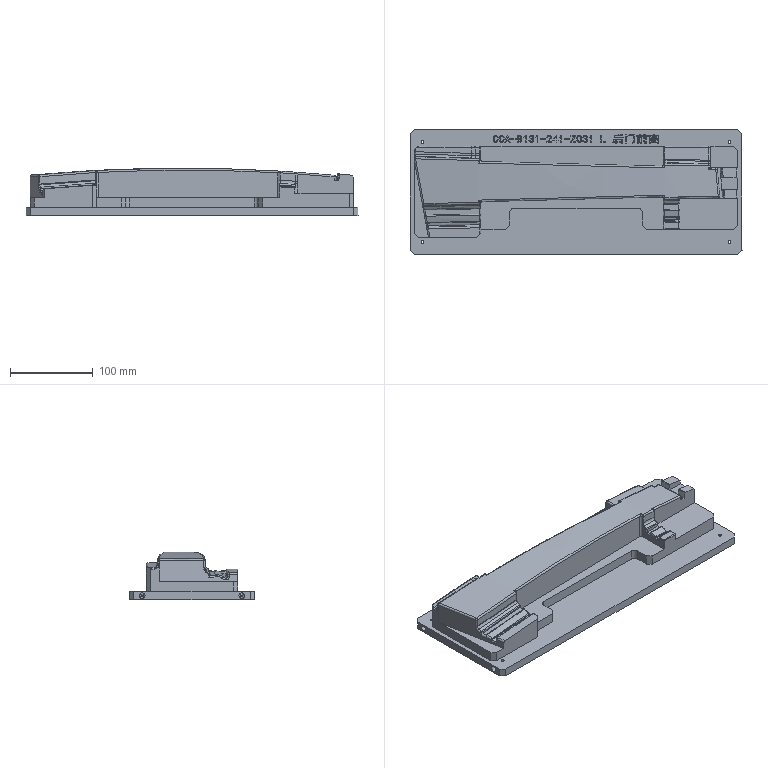NC program | NX | posted with a generic post | part box 400 x 150 x 57.494 mm
Lines 14042 to 16235 of 16235, first 2095 of 2182 lines:
(B3 , TOOL : D10)
N28076 M6
N28078 G54
N28080 G17 G0 G90 X-94.5 Y-54.975 S3500 M3
N28082 G43 Z69.994 H0
N28084 Y-54.994 Z24.994
N28086 G94 G1 Y-54.995 Z21.994 F1000.
N28088 Y-44.995 Z21.99
N28090 X-109.
N28092 Y-17.587 Z21.978
N28094 X99. Y-12.141 Z21.976
N28096 Y-43.995 Z21.989
N28098 X98.988 Y-44.499 Z21.99
N28100 X99.072 Y-44.995
N28102 X85.
N28104 X80. Y-39.995 Z21.988
N28106 Y-19.995 Z21.979
N28108 X84.348 Y-17.526 Z21.978
N28110 X94. Y-17.273
N28112 Y-39.995 Z21.988
N28114 X87.071
N28116 X85. Y-37.924 Z21.987
N28118 Y-19.995 Z21.979
N28120 X84.956 Y-19.133
N28122 X84.735 Y-18.297
N28124 X84.348 Y-17.526 Z21.978
N28126 X89.5 Y-21.893 Z21.98
N28128 Y-35.495 Z21.986
N28130 Y-21.893 Z21.98
N28132 X84.348 Y-17.526 Z21.978
N28134 X80. Y-19.995 Z21.979
N28136 X-80.
N28138 Y-39.995 Z21.988
N28140 X-85. Y-44.995 Z21.99
N28142 X-94.5
N28144 Y-39.995 Z21.988
N28146 X-104.
N28148 Y-22.458 Z21.98
N28150 X-85. Y-21.961
N28152 Y-37.924 Z21.987
N28154 X-87.071 Y-39.995 Z21.988
N28156 X-94.5
N28158 Y-34.995 Z21.986
N28160 X-99.
N28162 Y-27.329 Z21.982
N28164 X-90. Y-27.093
N28166 Y-34.995 Z21.986
N28168 X-94.5
N28170 Y-54.995 Z21.994
N28172 Y-54.994 Z24.994
N28174 G0 Y-54.975 Z69.994
(B4 , TOOL : D10)
N28176 X163.
N28178 Y-54.992 Z29.994
N28180 G1 Y-54.993 Z26.994
N28182 Y-44.993 Z26.99
N28184 X130.928
N28186 X131.012 Y-44.496
N28188 X131. Y-43.993 Z26.989
N28190 Y-13.371 Z26.977
N28192 X195.
N28194 Y-39.993 Z26.988
N28196 X190. Y-44.993 Z26.99
N28198 X163.
N28200 Y-39.993 Z26.988
N28202 X136.
N28204 Y-18.371 Z26.979
N28206 X190.
N28208 Y-37.922 Z26.987
N28210 X187.929 Y-39.993 Z26.988
N28212 X163.
N28214 Y-34.993 Z26.986
N28216 X141.
N28218 Y-23.371 Z26.981
N28220 X185.
N28222 Y-34.993 Z26.986
N28224 X163.
N28226 Y-29.993 Z26.984
N28228 X146.
N28230 Y-28.371 Z26.983
N28232 X180.
N28234 Y-29.993 Z26.984
N28236 X163.
N28238 Y-54.993 Z26.994
N28240 Y-54.992 Z29.994
N28242 G0 Y-54.975 Z69.994
(B5 , TOOL : D10)
N28244 X-205. Y-45.746
N28246 Z69.99
N28248 Y-45.765 Z24.99
N28250 G1 Y-45.766 Z21.99
N28252 X-195.
N28254 Y6.162 Z21.969
N28256 X-183.802 Y-54.995 Z21.994
N28258 X-190.
N28260 X-195. Y-49.995 Z21.992
N28262 Y-45.766 Z21.99
N28264 X-190.5
N28266 Y-43.4 Z21.989
N28268 X-189.44 Y-49.191 Z21.991
N28270 X-190.5 Y-48.131
N28272 Y-45.766 Z21.99
N28274 X-205.
N28276 Y-45.765 Z24.99
N28278 G0 Y-45.746 Z69.99
(B6 , TOOL : D10)
N28280 X181.5 Y65.146
N28282 Z69.944
N28284 Y65.132 Z35.444
N28286 G1 Y65.131 Z32.444
N28288 Y55.131 Z32.449
N28290 X190.
N28292 X195. Y50.131 Z32.451
N28294 Y35.131 Z32.457
N28296 X168.
N28298 Y53.131 Z32.449
N28300 X168.002 Y53.806
N28302 X167.916 Y54.477
N28304 X167.746 Y55.131
N28306 X181.5
N28308 Y50.131 Z32.451
N28310 X187.929
N28312 X190. Y48.06 Z32.452
N28314 Y40.131 Z32.455
N28316 X173.
N28318 Y50.131 Z32.451
N28320 X181.5
N28322 Y45.131 Z32.453
N28324 X185.
N28326 X178.
N28328 X181.5
N28330 Y65.131 Z32.444
N28332 Y65.132 Z35.444
N28334 G0 Y65.146 Z69.944
(B7 , TOOL : D10)
N28336 X-5.
N28338 Y65.132 Z35.444
N28340 G1 Y65.131 Z32.444
N28342 Y55.131 Z32.449
N28344 X99.254
N28346 X99.084 Y54.477
N28348 X98.998 Y53.806
N28350 X99. Y53.131
N28352 Y37.155 Z32.456
N28354 X-109. Y42.601 Z32.454
N28356 Y53.131 Z32.449
N28358 X-108.998 Y53.806
N28360 X-109.084 Y54.477
N28362 X-109.254 Y55.131
N28364 X-5.
N28366 Y50.131 Z32.451
N28368 X94.
N28370 Y42.287 Z32.454
N28372 X-104. Y47.472 Z32.452
N28374 Y50.131 Z32.451
N28376 X-5.
N28378 Y65.131 Z32.444
N28380 Y65.132 Z35.444
N28382 G0 Y65.146 Z69.944
N28384 M5
(B8 , TOOL : D4)
N28386 M6
N28388 G54
N28390 G17 G0 G90 X23.033 Y-12.116 S4000 M3
N28392 G43 Z69.976 H0
N28394 Z57.854
N28396 G94 G1 Z54.854 F1800.
N28398 G3 X20.981 Y-10.169 R2.
N28400 G1 X-37.755 Y-11.707
N28402 G3 X-39.702 Y-13.758 R2.
N28404 G1 Z57.854
N28406 G0 Z69.977
N28408 X-55.353 Y-14.169
N28410 Z57.555
N28412 G1 Z54.555
N28414 G2 X-53.406 Y-12.117 R2.
N28416 G1 X36.503 Y-9.763
N28418 X47.348 Y-9.479 Z54.257
N28420 X-64.793 Y-12.415
N28422 X-74.201 Y-12.662 Z53.958
N28424 X57.298 Y-9.218
N28426 X65.572 Y-9.002 Z53.659
N28428 X-82.458 Y-12.878
N28430 X-82.698 Y-12.884 Z53.65
N28432 X-82.937 Y-12.89 Z53.64
N28434 X-83.177 Y-12.897 Z53.63
N28436 X-83.416 Y-12.903 Z53.621
N28438 X-83.655 Y-12.909 Z53.611
N28440 X-83.895 Y-12.916 Z53.601
N28442 X-84.134 Y-12.922 Z53.592
N28444 X-84.374 Y-12.928 Z53.582
N28446 X-84.613 Y-12.935 Z53.572
N28448 X-84.853 Y-12.941 Z53.563
N28450 X-89.881 Y-13.073 Z53.36
N28452 X72.984 Y-8.808
N28454 X78.783 Y-8.656 Z53.104
N28456 X79.025 Y-8.65 Z53.094
N28458 X79.508 Y-8.637 Z53.072
N28460 X79.75 Y-8.631 Z53.062
N28462 X-96.64 Y-13.25
N28464 X-96.883 Y-13.256 Z53.05
N28466 X-97.126 Y-13.262 Z53.039
N28468 X-97.369 Y-13.269 Z53.027
N28470 X-97.612 Y-13.275 Z53.016
N28472 X-97.855 Y-13.281 Z53.004
N28474 X-98.098 Y-13.288 Z52.993
N28476 X-98.342 Y-13.294 Z52.981
N28478 X-98.585 Y-13.301 Z52.97
N28480 X-98.828 Y-13.307 Z52.958
N28482 X-102.961 Y-13.415 Z52.763
N28484 X86.043 Y-8.466
N28486 X90.539 Y-8.348 Z52.536
N28488 X90.775 Y-8.342 Z52.524
N28490 X91.485 Y-8.324 Z52.488
N28492 X91.722 Y-8.317 Z52.476
N28494 X91.958 Y-8.311 Z52.464
N28496 X-108.853 Y-13.57
N28498 X-113.011 Y-13.679 Z52.165
N28500 X97.552 Y-8.165
N28502 X97.794 Y-8.159 Z52.152
N28504 X98.035 Y-8.152 Z52.138
N28506 X98.277 Y-8.146 Z52.125
N28508 X98.76 Y-8.133 Z52.097
N28510 X99.002 Y-8.127 Z52.084
N28512 X99.244 Y-8.121 Z52.07
N28514 X99.969 Y-8.102 Z52.03
N28516 X100.211 Y-8.095 Z52.016
N28518 X100.452 Y-8.089 Z52.002
N28520 X101.177 Y-8.07 Z51.962
N28522 X101.419 Y-8.064 Z51.948
N28524 X101.661 Y-8.057 Z51.934
N28526 X102.628 Y-8.032 Z51.88
N28528 X102.869 Y-8.026 Z51.867
N28530 X-112.998 Y-13.679
N28532 Z51.568
N28534 X103. Y-8.023
N28536 Y-8.083
N28538 Z51.269
N28540 Y-8.023
N28542 X-112.998 Y-13.679
N28544 Z50.97
N28546 X103. Y-8.023
N28548 Y-8.083
N28550 Z50.671
N28552 Y-8.023
N28554 X-112.998 Y-13.679
N28556 Z50.373
N28558 X103. Y-8.023
N28560 Y-8.084
N28562 Z50.074
N28564 Y-8.023
N28566 X-112.998 Y-13.679
N28568 Z49.775
N28570 X103. Y-8.023
N28572 Y-8.084
N28574 Z49.476
N28576 Y-8.023
N28578 X-112.998 Y-13.68
N28580 Z49.178
N28582 X103. Y-8.024
N28584 Y-8.084
N28586 Z48.879
N28588 Y-8.024
N28590 X-112.998 Y-13.68
N28592 Z48.58
N28594 X103. Y-8.024
N28596 Y-8.084
N28598 Z48.281
N28600 Y-8.024
N28602 X-112.998 Y-13.68
N28604 Z47.983
N28606 X103. Y-8.024
N28608 Y-8.085
N28610 Z47.684
N28612 Y-8.024
N28614 X-112.998 Y-13.68
N28616 Z47.385
N28618 X103. Y-8.024
N28620 Y-8.085
N28622 Z47.086
N28624 Y-8.024
N28626 X-112.998 Y-13.68
N28628 Y-13.681 Z46.787
N28630 X103. Y-8.025
N28632 Y-8.085
N28634 Z46.489
N28636 Y-8.025
N28638 X-112.998 Y-13.681
N28640 Z46.19
N28642 X103. Y-8.025
N28644 Y-8.085
N28646 Z45.891
N28648 Y-8.025
N28650 X-112.998 Y-13.681
N28652 Z45.592
N28654 X103. Y-8.025
N28656 Y-8.086
N28658 Z45.294
N28660 Y-8.025
N28662 X-112.998 Y-13.681
N28664 Z44.995
N28666 X103. Y-8.025
N28668 Y-8.086
N28670 Z44.696
N28672 Y-8.025
N28674 X-112.998 Y-13.681
N28676 Y-13.682 Z44.397
N28678 X103. Y-8.025
N28680 Y-8.086
N28682 Z44.099
N28684 Y-8.026
N28686 X-112.998 Y-13.682
N28688 Z43.8
N28690 X103. Y-8.026
N28692 Y-8.086
N28694 Z43.501
N28696 Y-8.026
N28698 X-112.998 Y-13.682
N28700 Z43.202
N28702 X103. Y-8.026
N28704 Y-8.087
N28706 Z42.904
N28708 Y-8.026
N28710 X-112.998 Y-13.682
N28712 Z42.605
N28714 X103. Y-8.026
N28716 Z42.306
N28718 X-112.998 Y-13.682
N28720 Y-13.683 Z42.007
N28722 X103. Y-8.026
N28724 Y-8.108 Z41.708
N28726 Y-8.027
N28728 X-112.998 Y-13.683
N28730 Z41.41
N28732 X103. Y-8.027
N28734 Y-8.152
N28736 Y-8.213 Z41.111
N28738 Y-8.027
N28740 X-112.998 Y-13.683
N28742 X-113. Y-13.791 Z40.812
N28744 Y-13.684
N28746 X-112.965 Y-13.682
N28748 X103. Y-8.027
N28750 Y-8.294
N28752 Y-8.393 Z40.513
N28754 Y-8.027
N28756 X-112.965 Y-13.682
N28758 X-113. Y-13.684
N28760 Y-13.915
N28762 Y-14.06 Z40.215
N28764 Y-13.684
N28766 X-112.965 Y-13.682
N28768 X103. Y-8.027
N28770 Y-8.516
N28772 Y-8.659 Z39.916
N28774 Y-8.027
N28776 X-112.965 Y-13.683
N28778 X-113. Y-13.684
N28780 Y-14.23
N28782 Y-14.426 Z39.617
N28784 Y-13.684
N28786 X-112.965 Y-13.683
N28788 X103. Y-8.027
N28790 Y-8.823
N28792 Y-9.02 Z39.318
N28794 Y-8.028
N28796 X-112.965 Y-13.683
N28798 X-113. Y-13.684
N28800 Y-14.658
N28802 Y-14.794 Z39.169
N28804 Y-14.929 Z39.02
N28806 Y-13.684
N28808 X-112.965 Y-13.683
N28810 X103. Y-8.028
N28812 Y-9.242
N28814 Y-9.373 Z38.87
N28816 Y-9.503 Z38.721
N28818 Y-8.028
N28820 X-112.965 Y-13.683
N28822 X-113. Y-13.684
N28824 Y-15.241
N28826 Y-15.419 Z38.571
N28828 Y-15.597 Z38.422
N28830 Y-13.684
N28832 X-112.965 Y-13.683
N28834 X103. Y-8.028
N28836 Y-9.806
N28838 Y-9.985 Z38.273
N28840 Y-10.164 Z38.123
N28842 Y-8.028
N28844 X-112.965 Y-13.683
N28846 X-113. Y-13.684
N28848 Y-16.005
N28850 Y-16.22 Z37.974
N28852 Y-16.434 Z37.824
N28854 Y-13.684
N28856 X-112.965 Y-13.683
N28858 X103. Y-8.028
N28860 Y-10.573
N28862 Y-10.791 Z37.675
N28864 Y-11.009 Z37.526
N28866 Y-8.028
N28868 X-113. Y-13.684
N28870 Y-16.893
N28872 Y-17.136 Z37.376
N28874 Y-17.38 Z37.227
N28876 Y-13.685
N28878 X103. Y-8.028
N28880 Y-11.468
N28882 Y-11.633 Z37.127
N28884 Y-11.798 Z37.028
N28886 Y-11.963 Z36.928
N28888 Y-8.029
N28890 X-113. Y-13.685
N28892 Y-17.905
N28894 Y-18.095 Z36.829
N28896 Y-18.285 Z36.729
N28898 Y-18.475 Z36.629
N28900 Y-13.685
N28902 X103. Y-8.029
N28904 Y-12.489
N28906 Y-12.682 Z36.53
N28908 Y-12.874 Z36.43
N28910 Y-13.066 Z36.331
N28912 Y-8.029
N28914 X-113. Y-13.685
N28916 Y-18.978
N28918 Y-19.199 Z36.032
N28920 Y-13.685
N28922 X103. Y-8.029
N28924 Y-13.694
N28926 Y-13.958 Z35.733
N28928 Y-8.029
N28930 X-113. Y-13.685
N28932 Y-19.29
N28934 Y-19.299 Z35.434
N28936 Y-13.685
N28938 X103. Y-8.029
N28940 Y-13.958
N28942 Z35.136
N28944 Y-8.029
N28946 X-113. Y-13.685
N28948 Y-19.299
N28950 Z34.837
N28952 Y-13.686
N28954 X103. Y-8.029
N28956 Y-13.958
N28958 Z34.538
N28960 Y-8.03
N28962 X-113. Y-13.686
N28964 Y-19.299
N28966 Z34.239
N28968 Y-13.686
N28970 X103. Y-8.03
N28972 Y-13.958
N28974 Z33.94
N28976 Y-8.03
N28978 X-113. Y-13.686
N28980 Y-19.3
N28982 Z33.642
N28984 Y-13.686
N28986 X103. Y-8.03
N28988 Y-13.959
N28990 Z33.343
N28992 Y-8.03
N28994 X-113. Y-13.686
N28996 Y-19.3
N28998 Z33.044
N29000 Y-13.686
N29002 X103. Y-8.03
N29004 Y-13.959
N29006 G2 X101.401 Y-15.918 R2.
N29008 G1 Z36.044
N29010 G0 Z69.978
N29012 X132.204 Y-11.356 Z69.976
N29014 Z53.074
N29016 G1 Z50.074
N29018 G3 X130.204 Y-9.362 R2.
N29020 G1 X126.851
N29022 Z49.775
N29024 X134.316
N29026 X134.549 Z49.758
N29028 X135.014 Z49.722
N29030 X135.247 Z49.705
N29032 X135.48 Z49.687
N29034 X135.712 Z49.67
N29036 X135.945 Z49.652
N29038 X136.178 Z49.635
N29040 X136.41 Z49.617
N29042 X136.643 Z49.599
N29044 X136.876 Z49.582
N29046 X137.108 Z49.564
N29048 X137.341 Z49.547
N29050 X137.574 Z49.529
N29052 X137.806 Z49.512
N29054 X138.039 Z49.494
N29056 X138.272 Z49.476
N29058 X126.851
N29060 Z49.178
N29062 X142.144
N29064 X142.381 Z49.159
N29066 X142.617 Z49.14
N29068 X142.853 Z49.122
N29070 X143.089 Z49.103
N29072 X143.326 Z49.084
N29074 X143.562 Z49.066
N29076 X143.798 Z49.047
N29078 X144.035 Z49.028
N29080 X144.271 Z49.01
N29082 X144.507 Z48.991
N29084 X144.744 Z48.972
N29086 X144.98 Z48.954
N29088 X145.216 Z48.935
N29090 X145.452 Z48.916
N29092 X145.689 Z48.898
N29094 X145.925 Z48.879
N29096 X126.851
N29098 Y-9.363 Z48.58
N29100 X149.593
N29102 X149.832 Z48.56
N29104 X150.311 Z48.52
N29106 X150.55 Z48.5
N29108 X150.79 Z48.481
N29110 X151.029 Z48.461
N29112 X151.268 Z48.441
N29114 X151.508 Z48.421
N29116 X151.747 Z48.401
N29118 X151.986 Z48.381
N29120 X152.226 Z48.361
N29122 X152.465 Z48.341
N29124 X152.704 Y-9.362 Z48.321
N29126 X152.944 Y-9.363 Z48.301
N29128 X153.183 Z48.281
N29130 X126.851
N29132 Z47.983
N29134 X156.705
N29136 X156.933 Z47.963
N29138 X157.162 Z47.943
N29140 X157.391 Z47.923
N29142 X157.62 Z47.903
N29144 X157.848 Z47.883
N29146 X158.077 Z47.863
N29148 X158.306 Z47.843
N29150 X158.534 Z47.823
N29152 X158.763 Z47.803
N29154 X158.992 Z47.783
N29156 X159.221 Z47.763
N29158 X159.449 Z47.744
N29160 X159.678 Z47.724
N29162 X159.907 Z47.704
N29164 X160.136 Z47.684
N29166 X126.851
N29168 Z47.385
N29170 X163.529
N29172 X164.468 Z47.3
N29174 X164.702 Z47.278
N29176 X164.937 Z47.257
N29178 X165.172 Z47.236
N29180 X165.407 Z47.214
N29182 X165.642 Z47.193
N29184 X165.876 Z47.172
N29186 X166.111 Z47.15
N29188 X166.346 Z47.129
N29190 X166.581 Z47.108
N29192 X166.816 Z47.086
N29194 X126.851
N29196 Z46.787
N29198 X170.071
N29200 X171.169 Z46.489
N29202 X126.851
N29204 X126.85 Y-9.364 Z46.19
N29206 X171.169
N29208 Z45.891
N29210 X126.85
N29212 Z45.592
N29214 X171.169
N29216 Z45.294
N29218 X126.85
N29220 Z44.995
N29222 X171.169
N29224 Z44.696
N29226 X126.85
N29228 Z44.397
N29230 X171.169
N29232 Z44.099
N29234 X126.85
N29236 Y-9.365 Z43.8
N29238 X171.169
N29240 Z43.501
N29242 X126.85
N29244 Z43.202
N29246 X171.169
N29248 Z42.904
N29250 X126.85
N29252 G3 X126.963 Y-11.897 R2.
N29254 G1 Z45.904
N29256 G0 Z69.976
N29258 X184.781 Y-10.839
N29260 Z52.775
N29262 G1 Z49.775
N29264 G3 X182.851 Y-9.362 R2.
N29266 G1 X178.752
N29268 X178.563 Z49.476
N29270 X185.85
N29272 G2 X187.782 Y-10.847 R2.
N29274 G1 Z52.476
N29276 G0 Z69.976
N29278 X190.746 Y-10.854
N29280 Z52.178
N29282 G1 Z49.178
N29284 G3 X188.812 Y-9.362 R2.
N29286 G1 X178.477
N29288 X178.398 Z48.879
N29290 X191.737
N29292 X193.16 Y-9.363 Z48.58
N29294 X178.319
N29296 X178.241 Z48.281
N29298 X193.43
N29300 X193.565 Z48.132
N29302 X193.699 Z47.983
N29304 X178.162
N29306 X178.084 Z47.684
N29308 X193.969
N29310 X194.104 Z47.534
N29312 X194.238 Z47.385
N29314 X178.005
N29316 X177.927 Z47.086
N29318 X194.508
N29320 X194.643 Z46.937
N29322 X194.778 Z46.787
N29324 X177.848
N29326 X177.769 Z46.489
N29328 X195.
N29330 Y-9.364 Z46.19
N29332 X177.691
N29334 X177.612 Z45.891
N29336 X195.
N29338 Z45.592
N29340 X177.534
N29342 X177.455 Z45.294
N29344 X195.
N29346 Z44.995
N29348 X177.376
N29350 X177.298 Z44.696
N29352 X195.
N29354 Z44.397
N29356 X177.219
N29358 X177.141 Z44.099
N29360 X195.
N29362 Y-9.365 Z43.8
N29364 X177.062
N29366 X176.984 Z43.501
N29368 X195.
N29370 Z43.202
N29372 X176.905
N29374 X176.826 Z42.904
N29376 X195.
N29378 Z42.605
N29380 X176.748
N29382 G2 X175.491 Y-8.921 R2.018
N29384 G1 X174.212 Y-9.339
N29386 X173.892 Y-9.365
N29388 X126.85
N29390 X126.849 Z42.306
N29392 X195.
N29394 Z42.007
N29396 X126.849
N29398 Z41.708
N29400 X195.
N29402 Y-9.366 Z41.41
N29404 X126.832
N29406 X126.837 Z41.111
N29408 X195.
N29410 Z40.812
N29412 X126.854
N29414 Z40.513
N29416 X195.
N29418 Z40.215
N29420 X126.863
N29422 X126.904 Z39.916
N29424 X195.
N29426 Z39.617
N29428 X126.918
N29430 X126.96 Z39.318
N29432 X195.
N29434 Y-9.367 Z39.02
N29436 X127.065
N29438 X126.979 Y-9.37
N29440 X126.954 Y-9.462 Z38.721
N29442 X126.996 Y-9.367
N29444 X195.
N29446 Z38.422
N29448 X127.
N29450 Z38.123
N29452 X195.
N29454 Z37.824
N29456 X127.
N29458 Z37.526
N29460 X195.
N29462 Z37.227
N29464 X127.
N29466 Y-9.554 Z37.078
N29468 Y-9.741 Z36.928
N29470 Y-9.38
N29472 X127.005 Y-9.367
N29474 X195.
N29476 Z36.629
N29478 X127.005
N29480 X127. Y-9.381
N29482 Y-10.156
N29484 Y-10.374 Z36.48
N29486 Y-10.592 Z36.331
N29488 Y-9.381
N29490 X127.005 Y-9.368
N29492 X195.
N29494 Z36.032
N29496 X127.005
N29498 X127. Y-9.381
N29500 Y-11.06
N29502 Y-11.224 Z35.932
N29504 Y-11.389 Z35.833
N29506 Y-11.554 Z35.733
N29508 Y-9.381
N29510 X127.005 Y-9.368
N29512 X195.
N29514 Z35.434
N29516 X127.005
N29518 X127. Y-9.381
N29520 Y-12.092
N29522 Y-12.285 Z35.335
N29524 Y-12.478 Z35.235
N29526 Y-12.671 Z35.136
N29528 Y-9.381
N29530 X127.005 Y-9.368
N29532 X195.
N29534 Z34.837
N29536 X127.005
N29538 X127. Y-9.381
N29540 Y-13.307
N29542 Y-13.487 Z34.538
N29544 Y-9.382
N29546 X127.005 Y-9.368
N29548 X195.
N29550 Z34.239
N29552 X127.005
N29554 X127. Y-9.382
N29556 Y-13.487
N29558 Z33.94
N29560 Y-9.382
N29562 X127.006 Y-9.369
N29564 X195.
N29566 Z33.642
N29568 X127.006
N29570 X127. Y-9.382
N29572 Y-13.487
N29574 Z33.343
N29576 Y-9.382
N29578 X127.006 Y-9.369
N29580 X195.
N29582 Z33.044
N29584 X127.006
N29586 X127. Y-9.382
N29588 Y-13.487
N29590 Z32.745
N29592 Y-9.382
N29594 X127.006 Y-9.369
N29596 X195.
N29598 Z32.447
N29600 X127.006
N29602 X127. Y-9.382
N29604 Y-13.487
N29606 Z32.148
N29608 Y-9.383
N29610 X127.006 Y-9.369
N29612 X195.
N29614 Z31.849
N29616 X127.006
N29618 X127. Y-9.383
N29620 Y-13.488
N29622 Z31.55
N29624 Y-9.383
N29626 X127.006 Y-9.37
N29628 X195.
N29630 Z31.252
N29632 X127.006
N29634 X127. Y-9.383
N29636 Y-13.488
N29638 Z30.953
N29640 Y-9.383
N29642 X127.006 Y-9.37
N29644 X195.
N29646 Z30.654
N29648 X127.006
N29650 X127. Y-9.383
N29652 Y-13.488
N29654 G3 X128.977 Y-15.488 R2.
N29656 G1 Z33.654
N29658 G0 Z69.978
N29660 X-188.408 Y-16.864
N29662 Z50.086
N29664 G1 Z47.086
N29666 G3 X-187.126 Y-14.625 R2.
N29668 G1 X-196.967 Y39.125
N29670 Z46.787
N29672 X-187.126 Y-14.625
N29674 Z46.489
N29676 X-196.967 Y39.125
N29678 Z46.19
N29680 X-187.126 Y-14.625
N29682 Z45.891
N29684 X-196.967 Y39.125
N29686 Z45.592
N29688 X-187.126 Y-14.625
N29690 Z45.294
N29692 X-196.967 Y39.125
N29694 Z44.995
N29696 X-187.126 Y-14.626
N29698 Z44.696
N29700 X-196.967 Y39.124
N29702 Z44.397
N29704 X-187.126 Y-14.626
N29706 Z44.099
N29708 X-196.967 Y39.124
N29710 Z43.8
N29712 X-187.126 Y-14.626
N29714 Z43.501
N29716 X-196.967 Y39.124
N29718 Z43.202
N29720 X-187.126 Y-14.626
N29722 Z42.904
N29724 X-196.967 Y39.124
N29726 Z42.605
N29728 X-187.126 Y-14.627
N29730 Z42.306
N29732 X-196.967 Y39.123
N29734 Z42.007
N29736 X-187.126 Y-14.627
N29738 Z41.708
N29740 X-196.967 Y39.123
N29742 Z41.41
N29744 X-187.126 Y-14.627
N29746 Z41.111
N29748 X-196.967 Y39.123
N29750 Z40.812
N29752 X-187.126 Y-14.627
N29754 Z40.513
N29756 X-196.967 Y39.123
N29758 Z40.215
N29760 X-187.126 Y-14.628
N29762 Z39.916
N29764 X-196.967 Y39.122
N29766 Z39.617
N29768 X-187.126 Y-14.628
N29770 Z39.318
N29772 X-196.967 Y39.122
N29774 Z39.02
N29776 X-187.126 Y-14.628
N29778 Z38.721
N29780 X-196.967 Y39.122
N29782 Z38.422
N29784 X-187.126 Y-14.628
N29786 X-187.127 Y-14.619 Z38.123
N29788 X-196.967 Y39.122
N29790 Z37.824
N29792 X-187.13 Y-14.607
N29794 X-187.129 Y-14.609 Z37.526
N29796 X-196.967 Y39.121
N29798 Z37.227
N29800 X-187.126 Y-14.628
N29802 X-187.12 Y-14.658 Z36.928
N29804 X-196.967 Y39.121
N29806 Z36.629
N29808 X-187.112 Y-14.702
N29810 X-187.101 Y-14.764 Z36.331
N29812 X-196.967 Y39.121
N29814 Z36.032
N29816 X-187.087 Y-14.84
N29818 X-187.071 Y-14.929 Z35.733
N29820 X-196.967 Y39.121
N29822 Z35.434
N29824 X-187.051 Y-15.039
N29826 X-187.028 Y-15.162 Z35.136
N29828 X-196.967 Y39.12
N29830 Z34.837
N29832 X-187.001 Y-15.309
N29834 X-186.971 Y-15.472 Z34.538
N29836 X-196.967 Y39.12
N29838 Z34.239
N29840 X-186.936 Y-15.663
N29842 X-186.898 Y-15.874 Z33.94
N29844 X-196.967 Y39.12
N29846 Z33.642
N29848 X-186.853 Y-16.119
N29850 X-186.828 Y-16.258 Z33.492
N29852 X-186.802 Y-16.398 Z33.343
N29854 X-196.967 Y39.12
N29856 Z33.044
N29858 X-186.744 Y-16.715
N29860 X-186.707 Y-16.896 Z32.945
N29862 X-186.669 Y-17.076 Z32.845
N29864 X-186.641 Y-17.259 Z32.745
N29866 X-186.678 Y-17.074
N29868 X-196.967 Y39.119
N29870 Z32.447
N29872 X-186.608 Y-17.458
N29874 X-186.567 Y-17.684 Z32.297
N29876 X-186.525 Y-17.91 Z32.148
N29878 X-196.967 Y39.119
N29880 Z31.849
N29882 X-186.442 Y-18.364
N29884 X-186.413 Y-18.526 Z31.749
N29886 X-186.383 Y-18.688 Z31.65
N29888 X-186.353 Y-18.85 Z31.55
N29890 X-196.967 Y39.119
N29892 Z31.252
N29894 X-186.257 Y-19.373
N29896 X-186.223 Y-19.561 Z31.152
N29898 X-186.188 Y-19.75 Z31.052
N29900 X-186.154 Y-19.938 Z30.953
N29902 X-196.967 Y39.119
N29904 Z30.654
N29906 X-186.064 Y-20.427
N29908 Z30.355
N29910 X-196.967 Y39.119
N29912 Y39.118 Z30.056
N29914 X-186.064 Y-20.427
N29916 Z29.758
N29918 X-196.967 Y39.118
N29920 Z29.459
N29922 X-186.064 Y-20.428
N29924 Z29.16
N29926 X-196.967 Y39.118
N29928 Z28.861
N29930 X-186.064 Y-20.428
N29932 Z28.563
N29934 X-196.967 Y39.118
N29936 Z28.264
N29938 X-186.064 Y-20.428
N29940 Z27.965
N29942 X-196.967 Y39.118
N29944 Y39.117 Z27.666
N29946 X-186.064 Y-20.428
N29948 G2 X-187.631 Y-22.748 R2.
N29950 G1 Z30.666
N29952 G0 Z69.981
N29954 X-111.311 Y41.83 Z69.954
N29956 Z47.995
N29958 G1 Z44.995
N29960 G3 X-113. Y39.854 R2.
N29962 G1 Y38.748
N29964 X-113.003 Y38.71
N29966 X-112.965 Y38.712
N29968 X-112.871 Y38.709
N29970 Z44.696
N29972 X-112.965 Y38.712
N29974 X-113.003 Y38.71
N29976 X-113. Y38.748
N29978 Y40.213
N29980 Y40.432 Z44.547
N29982 Y40.65 Z44.397
N29984 Y38.748
N29986 X-113.003 Y38.71
N29988 X-112.965 Y38.712
N29990 X-112.871 Y38.709
N29992 Z44.099
N29994 X-112.965 Y38.712
N29996 X-113.003 Y38.71
N29998 X-113. Y38.748
N30000 Y41.207
N30002 X-113.001 Y41.407 Z44.024
N30004 Y41.607 Z43.949
N30006 Y41.807 Z43.874
N30008 X-113. Y42.007 Z43.8
N30010 Y38.748
N30012 X-113.003 Y38.71
N30014 X-112.965 Y38.712
N30016 X-112.871 Y38.709
N30018 Z43.501
N30020 X-112.965 Y38.712
N30022 X-113.003 Y38.71
N30024 X-113. Y38.748
N30026 Y53.148
N30028 G3 X-113.059 Y53.81 R3.733
N30030 G1 X-113.104 Y54.031 Z43.471
N30032 X-113.161 Y54.255 Z43.441
N30034 X-113.235 Y54.479 Z43.411
N30036 X-113.322 Y54.703 Z43.382
N30038 X-113.426 Y54.92 Z43.352
N30040 X-113.537 Y55.134 Z43.322
N30042 X-113.665 Y55.336 Z43.292
N30044 X-113.798 Y55.531 Z43.262
N30046 X-113.942 Y55.711 Z43.232
N30048 X-114.091 Y55.878 Z43.202
N30050 G2 X-113.489 Y55.052 R3.666
N30052 X-113. Y53.135 R4.055
N30054 G1 Y38.748
N30056 X-113.003 Y38.71
N30058 X-112.965 Y38.712
N30060 X-112.871 Y38.709
N30062 Z42.904
N30064 X-112.964 Y38.712
N30066 X-113.003 Y38.71
N30068 X-113. Y38.748
N30070 Y53.135
N30072 G3 X-114.334 Y56.119 R3.898
N30074 G1 X-114.336 Y56.116 Z42.605
N30076 G2 X-113. Y53.135 R3.994
N30078 G1 Y38.748
N30080 X-113.003 Y38.71
N30082 X-112.964 Y38.712
N30084 X-112.871 Y38.709
N30086 Z42.306
N30088 X-112.964 Y38.712
N30090 X-113.003 Y38.71
N30092 X-113. Y38.749
N30094 Y53.135
N30096 G3 X-114.337 Y56.115 R4.007
N30098 G1 Y56.116 Z42.007
N30100 G2 X-113. Y53.135 R4.007
N30102 G1 Y38.749
N30104 X-113.003 Y38.71
N30106 X-112.964 Y38.712
N30108 X-112.87 Y38.709
N30110 Z41.708
N30112 X-112.964 Y38.712
N30114 X-113.003 Y38.71
N30116 X-113. Y38.749
N30118 Y53.135
N30120 G3 X-114.337 Y56.116 R4.007
N30122 G1 Z41.41
N30124 G2 X-113. Y53.134 R4.007
N30126 G1 Y38.749
N30128 X-113.003 Y38.71
N30130 X-112.964 Y38.712
N30132 X-112.87 Y38.709
N30134 Z41.111
N30136 X-112.964 Y38.712
N30138 X-113.003 Y38.71
N30140 X-113. Y38.749
N30142 Y53.134
N30144 G3 X-114.337 Y56.116 R4.007
N30146 G1 Z40.812
N30148 G2 X-113. Y53.134 R4.007
N30150 G1 Y38.749
N30152 X-113.003 Y38.71
N30154 X-112.964 Y38.712
N30156 X-112.87 Y38.709
N30158 Z40.513
N30160 X-112.964 Y38.712
N30162 X-113.003 Y38.71
N30164 X-113. Y38.749
N30166 Y53.134
N30168 G3 X-114.337 Y56.116 R4.007
N30170 G1 X-114.336 Z40.215
N30172 G2 X-113. Y53.134 R4.004
N30174 G1 Y38.749
N30176 X-113.003 Y38.71
N30178 X-112.964 Y38.712
N30180 X-112.87 Y38.709
N30182 Z39.916
N30184 X-112.963 Y38.712
N30186 X-113.003 Y38.71
N30188 X-113. Y38.749
N30190 Y53.134
N30192 G3 X-114.336 Y56.116 R4.004
N30194 G1 Z39.617
N30196 G2 X-113. Y53.134 R4.004
N30198 G1 Y38.75
N30200 X-113.003 Y38.71
N30202 X-112.963 Y38.712
N30204 X-112.87 Y38.709
N30206 Z39.318
N30208 X-112.963 Y38.712
N30210 X-113.003 Y38.71
N30212 X-113. Y38.75
N30214 Y53.134
N30216 G3 X-114.336 Y56.116 R4.004
N30218 G1 Z39.02
N30220 G2 X-113. Y53.134 R4.004
N30222 G1 Y38.75
N30224 X-113.003 Y38.71
N30226 X-112.963 Y38.712
N30228 X-112.87 Y38.709
N30230 Y38.71 Z38.721
N30232 X-112.963 Y38.712
N30234 X-113.003 Y38.71
N30236 X-113. Y38.75
N30238 Y53.133
N30240 G3 X-114.336 Y56.116 R4.004
N30242 G1 Z38.422
N30244 G2 X-113. Y53.133 R4.004
N30246 G1 Y38.75
N30248 X-113.003 Y38.71
N30250 X-112.963 Y38.712
N30252 X-112.87 Y38.71
N30254 Z38.123
N30256 X-112.963 Y38.712
N30258 X-113.003 Y38.71
N30260 X-113. Y38.75
N30262 Y53.133
N30264 G3 X-114.336 Y56.116 R4.004
N30266 G1 Z37.824
N30268 G2 X-113. Y53.133 R4.003
N30270 G1 Y38.75
N30272 X-113.003 Y38.71
N30274 X-112.963 Y38.712
N30276 X-112.87 Y38.71
N30278 Z37.526
N30280 X-112.963 Y38.712
N30282 X-113.003 Y38.71
N30284 X-113. Y38.75
N30286 Y53.133
N30288 G3 X-114.336 Y56.116 R4.003
N30290 G1 Y56.117 Z37.227
N30292 G2 X-113. Y53.133 R4.003
N30294 G1 Y38.75
N30296 X-113.003 Y38.71
N30298 X-112.962 Y38.712
N30300 X-112.87 Y38.71
N30302 Z36.928
N30304 X-112.962 Y38.712
N30306 X-113.003 Y38.71
N30308 X-113. Y38.751
N30310 Y53.133
N30312 G3 X-114.336 Y56.117 R4.003
N30314 G1 X-114.335 Z36.629
N30316 G2 X-113. Y53.133 R4.003
N30318 G1 Y38.751
N30320 X-113.003 Y38.71
N30322 X-112.962 Y38.712
N30324 X-112.87 Y38.71
N30326 Z36.331
N30328 X-112.962 Y38.712
N30330 X-113.003 Y38.71
N30332 X-113. Y38.751
N30334 Y53.132
N30336 G3 X-114.335 Y56.117 R4.003
N30338 G1 Z36.032
N30340 G2 X-113. Y53.132 R4.003
N30342 G1 Y38.751
N30344 X-113.003 Y38.71
N30346 X-112.962 Y38.712
N30348 X-112.87 Y38.71
N30350 Z35.733
N30352 X-112.962 Y38.712
N30354 X-113.003 Y38.71
N30356 X-113. Y38.751
N30358 Y53.132
N30360 G3 X-114.335 Y56.117 R4.003
N30362 G1 Z35.434
N30364 G2 X-113. Y53.132 R4.002
N30366 G1 Y38.751
N30368 X-113.003 Y38.71
N30370 X-112.962 Y38.712
N30372 X-112.87 Y38.71
N30374 Z35.136
N30376 X-112.962 Y38.712
N30378 X-113.003 Y38.71
N30380 X-113. Y38.751
N30382 Y53.132
N30384 G3 X-114.335 Y56.117 R4.002
N30386 G1 Z34.837
N30388 G2 X-113. Y53.132 R4.002
N30390 G1 Y38.751
N30392 X-113.003 Y38.71
N30394 X-112.962 Y38.712
N30396 X-112.87 Y38.71
N30398 Z34.538
N30400 X-112.963 Y38.712
N30402 X-113.003 Y38.71
N30404 X-113. Y38.75
N30406 Y53.132
N30408 G3 X-114.335 Y56.117 R4.002
N30410 G1 Z34.239
N30412 G2 X-113. Y53.132 R4.002
N30414 G1 Y38.75
N30416 X-113.003 Y38.71
N30418 X-112.963 Y38.712
N30420 X-112.87 Y38.71
N30422 Z33.94
N30424 X-112.963 Y38.712
N30426 X-113.003 Y38.71
N30428 X-113. Y38.75
N30430 Y53.131
N30432 G3 X-114.335 Y56.117 R4.002
N30434 G1 Z33.642
N30436 G2 X-113. Y53.131 R4.001
N30438 G1 Y38.75
N30440 X-113.003 Y38.71
N30442 X-112.963 Y38.712
N30444 X-112.87 Y38.71
N30446 Z33.343
N30448 X-112.963 Y38.712
N30450 X-113.003 Y38.71
N30452 X-113. Y38.75
N30454 Y53.131
N30456 G3 X-114.335 Y56.117 R4.001
N30458 G1 Z33.044
N30460 G2 X-113. Y53.131 R4.001
N30462 G1 Y38.75
N30464 X-113.003 Y38.71
N30466 X-112.963 Y38.712
N30468 X-112.87 Y38.71
N30470 Z32.745
N30472 X-112.963 Y38.712
N30474 X-113.003 Y38.71
N30476 X-113. Y38.75
N30478 Y53.131
N30480 G3 X-114.335 Y56.117 R4.001
N30482 G1 X-114.206 Y55.997 Z32.447
N30484 G2 X-113. Y53.131 R4.
N30486 G1 Y38.751
N30488 X-113.003 Y38.71
N30490 X-112.962 Y38.712
N30492 X-112.87 Y38.71
N30494 G3 X-110.819 Y40.657 R2.
N30496 G1 Z35.447
N30498 G0 Z69.955
N30500 X100.977 Y35.119 Z69.957
N30502 Z45.904
N30504 G1 Z42.904
N30506 G3 X102.924 Y33.068 R2.
N30508 G1 X103. Y33.066
N30510 Y34.241
N30512 Y34.455 Z42.754
N30514 Y34.669 Z42.605
N30516 Y33.066
N30518 X102.924 Y33.068
N30520 X102.923 Z42.306
N30522 X103. Y33.066
N30524 Y35.19
N30526 Y35.412 Z42.206
N30528 Y35.634 Z42.107
N30530 Y35.856 Z42.007
N30532 Y33.066
N30534 X102.923 Y33.068
N30536 Z41.708
N30538 X103. Y33.066
N30540 Y36.907
N30542 X103.002 Y37.152 Z41.702
N30544 X103.004 Y37.396 Z41.695
N30546 X103.007 Y37.641 Z41.689
N30548 X103.008 Y37.885 Z41.682
N30550 X103.009 Y38.13 Z41.675
N30552 X103.008 Y38.374 Z41.669
N30554 X103.007 Y38.619 Z41.662
N30556 Y38.863 Z41.655
N30558 X103.006 Y39.108 Z41.649
N30560 X103.007 Y39.352 Z41.642
N30562 X103.006 Y39.597 Z41.635
N30564 X103.007 Y39.841 Z41.629
N30566 X103.006 Y40.086 Z41.622
N30568 X103.005 Y40.33 Z41.615
N30570 Y40.575 Z41.609
N30572 X103.004 Y40.819 Z41.602
N30574 X103.005 Y41.064 Z41.596
N30576 X103.004 Y41.308 Z41.589
N30578 X103.003 Y41.553 Z41.582
N30580 X103.004 Y41.797 Z41.576
N30582 X103.003 Y42.041 Z41.569
N30584 Y42.286 Z41.562
N30586 Y42.53 Z41.556
N30588 Y42.775 Z41.549
N30590 X103.002 Y43.019 Z41.542
N30592 Y43.264 Z41.536
N30594 Y43.508 Z41.529
N30596 Y43.753 Z41.523
N30598 Y43.997 Z41.516
N30600 Y44.242 Z41.509
N30602 Y44.486 Z41.503
N30604 X103.001 Y44.731 Z41.496
N30606 Y44.975 Z41.489
N30608 Y45.22 Z41.483
N30610 Y45.464 Z41.476
N30612 Y45.709 Z41.469
N30614 Y45.953 Z41.463
N30616 Y46.198 Z41.456
N30618 Y46.442 Z41.449
N30620 Y46.687 Z41.443
N30622 Y46.931 Z41.436
N30624 X103. Y47.176 Z41.43
N30626 Y47.42 Z41.423
N30628 Y47.664 Z41.416
N30630 Y47.909 Z41.41
N30632 Y33.066
N30634 X102.923 Y33.068
N30636 Z41.111
N30638 X103. Y33.066
N30640 Y53.135
N30642 Z40.812
N30644 Y33.066
N30646 X102.923 Y33.068
N30648 Z40.513
N30650 X103. Y33.066
N30652 Y53.135
N30654 Z40.215
N30656 Y33.067
N30658 X102.923 Y33.069
N30660 Z39.916
N30662 X103. Y33.067
N30664 Y53.135
N30666 Z39.617
N30668 Y33.067
N30670 X102.923 Y33.069
N30672 Z39.318
N30674 X103. Y33.067
N30676 Y53.135
N30678 X103.005 Y53.355 Z39.297
N30680 X103.024 Y53.584 Z39.276
N30682 X103.06 Y53.82 Z39.254
N30684 X103.11 Y54.062 Z39.233
N30686 X103.176 Y54.305 Z39.212
N30688 X103.259 Y54.548 Z39.19
N30690 X103.358 Y54.787 Z39.169
N30692 X103.472 Y55.019 Z39.148
N30694 X103.6 Y55.241 Z39.126
N30696 X103.74 Y55.451 Z39.105
N30698 X103.889 Y55.647 Z39.084
N30700 X104.044 Y55.829 Z39.062
N30702 X104.204 Y55.994 Z39.041
N30704 X104.365 Y56.144 Z39.02
N30706 G3 X103. Y53.134 R4.001
N30708 G1 Y33.067
N30710 X102.923 Y33.069
N30712 Z38.721
N30714 X103. Y33.067
N30716 Y53.133
N30718 G2 X104.365 Y56.144 R4.001
N30720 G1 Z38.422
N30722 G3 X103. Y53.133 R4.001
N30724 G1 Y33.067
N30726 X102.923 Y33.069
N30728 Z38.123
N30730 X103. Y33.067
N30732 Y53.133
N30734 G2 X104.365 Y56.144 R4.001
N30736 G1 Z37.824
N30738 G3 X103. Y53.133 R4.002
N30740 G1 Y33.067
N30742 X102.923 Y33.069
N30744 Y33.07 Z37.526
N30746 X103. Y33.068
N30748 Y53.133
N30750 G2 X104.365 Y56.144 R4.002
N30752 G1 Z37.227
N30754 G3 X103. Y53.133 R4.002
N30756 G1 Y33.068
N30758 X102.923 Y33.07
N30760 Z36.928
N30762 X103. Y33.068
N30764 Y53.133
N30766 G2 X104.361 Y56.14 R4.002
N30768 G1 X104.356 Y56.136 Z36.629
N30770 G3 X103. Y53.133 R4.002
N30772 G1 Y33.068
N30774 X102.923 Y33.07
N30776 X102.922 Z36.331
N30778 X103. Y33.068
N30780 Y53.132
N30782 G2 X104.351 Y56.132 R4.002
N30784 G1 X104.346 Y56.127 Z36.032
N30786 G3 X103. Y53.132 R4.002
N30788 G1 Y33.068
N30790 X102.922 Y33.07
N30792 Z35.733
N30794 X103. Y33.068
N30796 Y53.132
N30798 G2 X104.34 Y56.122 R4.003
N30800 G1 X104.333 Y56.116 Z35.434
N30802 G3 X103. Y53.132 R4.003
N30804 G1 Y33.068
N30806 X102.922 Y33.07
N30808 Z35.136
N30810 X103. Y33.068
N30812 Y53.132
N30814 G2 X104.325 Y56.109 R4.003
N30816 G1 X104.316 Y56.1 Z34.837
N30818 G3 X103. Y53.132 R4.003
N30820 G1 Y33.069
N30822 X102.922 Y33.071
N30824 Z34.538
N30826 X103. Y33.069
N30828 Y53.132
N30830 G2 X104.303 Y56.088 R4.003
N30832 G1 Z34.239
N30834 G3 X103. Y53.132 R4.003
N30836 G1 Y33.069
N30838 X102.922 Y33.071
N30840 Z33.94
N30842 X103. Y33.069
N30844 Y53.131
N30846 G2 X104.303 Y56.088 R4.003
N30848 G1 X104.365 Y56.144 Z33.642
N30850 G3 X103. Y53.131 R4.003
N30852 G1 Y33.069
N30854 X102.922 Y33.071
N30856 Z33.343
N30858 X103. Y33.069
N30860 Y53.131
N30862 G2 X104.365 Y56.144 R4.004
N30864 G1 Z33.044
N30866 G3 X103. Y53.131 R4.004
N30868 G1 Y33.069
N30870 X102.922 Y33.071
N30872 Z32.745
N30874 X103. Y33.069
N30876 Y53.131
N30878 G2 X104.365 Y56.144 R4.004
N30880 G1 Z32.447
N30882 G3 X103. Y53.131 R4.004
N30884 G1 Y33.069
N30886 Z35.447
N30888 G0 Z69.958
N30890 X165.725 Y34.125 Z69.957
N30892 Z42.916
N30894 G1 Z39.916
N30896 G3 X164. Y32.144 R2.
N30898 G1 Y31.152
N30900 X164.096 Y31.137
N30902 Z39.617
N30904 X164. Y31.152
N30906 Y32.379
N30908 Y32.519 Z39.468
N30910 Y32.66 Z39.318
N30912 Y31.152
N30914 X164.096 Y31.137
N30916 Z39.02
N30918 X164. Y31.153
N30920 Y32.994
N30922 Y33.19 Z38.87
N30924 Y33.387 Z38.721
N30926 Y31.153
N30928 X164.096 Y31.137
N30930 Z38.422
N30932 X164. Y31.153
N30934 Y33.857
N30936 Y34.049 Z38.322
N30938 Y34.241 Z38.223
N30940 Y34.432 Z38.123
N30942 Y31.153
N30944 X164.096 Y31.137
N30946 Z37.824
N30948 X164. Y31.153
N30950 Y35.24
N30952 X163.998 Y35.472 Z37.803
N30954 X163.994 Y35.704 Z37.782
N30956 X163.992 Y35.936 Z37.76
N30958 X163.988 Y36.168 Z37.739
N30960 X163.986 Y36.4 Z37.718
N30962 X163.985 Y36.632 Z37.696
N30964 X163.987 Y36.864 Z37.675
N30966 X163.99 Y37.096 Z37.654
N30968 X163.993 Y37.328 Z37.632
N30970 X163.996 Y37.56 Z37.611
N30972 X163.997 Y37.792 Z37.59
N30974 X163.998 Y38.024 Z37.568
N30976 X163.999 Y38.256 Z37.547
N30978 X164. Y38.488 Z37.526
N30980 Y31.153
N30982 X164.096 Y31.137
N30984 Z37.227
N30986 X164. Y31.153
N30988 Y53.133
N30990 G3 X162.236 Y56.449 R4.
N30992 G1 Z36.928
N30994 G2 X164. Y53.133 R4.
N30996 G1 Y31.153
N30998 X164.096 Y31.137
N31000 Y31.138 Z36.629
N31002 X164. Y31.153
N31004 Y53.133
N31006 G3 X162.236 Y56.449 R4.
N31008 G1 Z36.331
N31010 G2 X164. Y53.132 R4.
N31012 G1 Y31.153
N31014 X164.096 Y31.138
N31016 Z36.032
N31018 X164. Y31.153
N31020 Y53.132
N31022 G3 X162.236 Y56.449 R4.
N31024 G1 Z35.733
N31026 G2 X164. Y53.132 R4.001
N31028 G1 Y31.154
N31030 X164.096 Y31.138
N31032 Z35.434
N31034 X164. Y31.154
N31036 Y53.132
N31038 G3 X162.236 Y56.449 R4.001
N31040 G1 Z35.136
N31042 G2 X164. Y53.132 R4.001
N31044 G1 Y31.154
N31046 X164.096 Y31.138
N31048 Z34.837
N31050 X164. Y31.154
N31052 Y53.132
N31054 G3 X162.236 Y56.449 R4.001
N31056 G1 Z34.538
N31058 G2 X164. Y53.132 R4.001
N31060 G1 Y31.154
N31062 X164.096 Y31.138
N31064 Z34.239
N31066 X164. Y31.154
N31068 Y53.132
N31070 G3 X162.236 Y56.449 R4.001
N31072 G1 Z33.94
N31074 G2 X164. Y53.131 R4.001
N31076 G1 Y31.154
N31078 X164.096 Y31.138
N31080 Z33.642
N31082 X164. Y31.154
N31084 Y53.131
N31086 G3 X162.236 Y56.449 R4.001
N31088 G1 Z33.343
N31090 G2 X164. Y53.131 R4.001
N31092 G1 Y31.154
N31094 X164.096 Y31.138
N31096 Z33.044
N31098 X164. Y31.154
N31100 Y53.131
N31102 G3 X162.236 Y56.449 R4.002
N31104 G1 Z32.745
N31106 G2 X164. Y53.131 R4.002
N31108 G1 Y31.155
N31110 X164.096 Y31.138
N31112 Z32.447
N31114 X164. Y31.155
N31116 Y53.131
N31118 G3 X162.236 Y56.449 R4.002
N31120 G2 X161.533 Y58.933 R2.
N31122 G1 Z35.447
N31124 G0 Z69.947
N31126 X-111.349 Y-40.618 Z69.988
N31128 Z38.733
N31130 G1 Z35.733
N31132 G3 X-113. Y-42.588 R2.
N31134 G1 Y-49.989
N31136 Y-49.99 Z35.434
N31138 Y-42.314
N31140 Y-42.199 Z35.136
N31142 Y-49.99
N31144 Z34.837
N31146 Y-42.176
N31148 Z34.538
N31150 Y-49.99
N31152 Z34.239
N31154 Y-42.176
N31156 Z33.94
N31158 Y-49.99
N31160 Z33.642
N31162 Y-42.176
N31164 Z33.343
N31166 Y-49.99
N31168 Y-49.991 Z33.044
N31170 Y-42.177
N31172 Z32.745
N31174 Y-49.991
N31176 Z32.447
N31178 Y-42.22
N31180 Y-42.19 Z32.148
N31182 Y-49.991
N31184 Z31.849
N31186 Y-42.189
N31188 Y-42.148 Z31.55
N31190 Y-49.991
N31192 Z31.252
N31194 Y-42.069
N31196 Y-41.947 Z30.953
N31198 Y-49.991
N31200 Y-49.992 Z30.654
N31202 Y-41.775
N31204 Y-41.532 Z30.355
N31206 Y-49.992
N31208 Z30.056
N31210 Y-41.192
N31212 G2 X-111.067 Y-39.193 R2.
N31214 G1 Z33.056
N31216 G0 Z69.987
N31218 X-111.4 Y-25.583 Z69.982
N31220 Z36.94
N31222 G1 Z33.94
N31224 G3 X-113. Y-27.543 R2.
N31226 G1 Y-29.09
N31228 Y-29.298 Z33.881
N31230 Y-29.507 Z33.821
N31232 Y-29.715 Z33.761
N31234 Y-29.923 Z33.701
N31236 Y-30.131 Z33.642
N31238 Y-27.543
N31240 Z33.343
N31242 Y-31.171
N31244 Y-31.379 Z33.283
N31246 Y-31.588 Z33.223
N31248 Y-31.796 Z33.164
N31250 Y-32.004 Z33.104
N31252 Y-32.212 Z33.044
N31254 Y-27.543
N31256 G2 X-111. Y-25.543 R2.
N31258 G1 Z36.044
N31260 G0 Z69.982
N31262 X101.401 Y-15.918 Z69.978
N31264 Z35.745
N31266 G1 Z32.745
N31268 G3 X103. Y-13.959 R2.
N31270 G1 Y-8.03
N31272 X-113. Y-13.686
N31274 Y-33.252
N31276 Y-34.241 Z32.447
N31278 Y-13.687
N31280 X103. Y-8.03
N31282 Y-13.959
N31284 Z32.148
N31286 Y-8.031
N31288 X-113. Y-13.687
N31290 Y-35.121
N31292 Z31.849
N31294 Y-13.687
N31296 X103. Y-8.031
N31298 Y-13.959
N31300 Z31.55
N31302 Y-8.031
N31304 X-113. Y-13.687
N31306 Y-35.121
N31308 Y-35.122 Z31.252
N31310 Y-13.687
N31312 X103. Y-8.031
N31314 Y-13.96
N31316 Z30.953
N31318 Y-8.031
N31320 X-113. Y-13.687
N31322 Y-35.122
N31324 X-113.005 Y-35.354 Z30.853
N31326 X-113.002 Y-35.587 Z30.754
N31328 X-113. Y-35.819 Z30.654
N31330 Y-13.687
N31332 X103. Y-8.031
N31334 Y-13.96
N31336 G2 X101.036 Y-15.959 R2.
N31338 G1 Z33.654
N31340 G0 Z69.978
N31342 X108. Y-48.99 Z69.991
N31344 Z36.94
N31346 G1 Z33.94
N31348 G3 X106. Y-46.99 R2.
N31350 G2 X103. Y-43.99 R3.
N31352 G1 Y-36.869
N31354 Z33.642
N31356 Y-43.99
N31358 G3 X106. Y-46.99 R3.
N31360 G1 Z33.343
N31362 G2 X103. Y-43.99 R3.
N31364 G1 Y-36.87
N31366 Z33.044
N31368 Y-43.991
N31370 G3 X106. Y-46.991 R3.
N31372 G1 Z32.745
N31374 G2 X103. Y-43.991 R3.
N31376 G1 Y-36.87
N31378 Z32.447
N31380 Y-43.991
N31382 G3 X106. Y-46.991 R3.
N31384 G1 Z32.148
N31386 G2 X103. Y-43.991 R3.
N31388 G1 Y-36.872
N31390 Y-36.886 Z31.849
N31392 Y-43.991
N31394 G3 X106. Y-46.991 R3.
N31396 G1 Z31.55
N31398 G2 X103. Y-43.991 R3.
N31400 G1 Y-36.865
N31402 Y-36.805 Z31.252
N31404 Y-43.991
N31406 G3 X106. Y-46.991 R3.
N31408 G1 Z30.953
N31410 G2 X103. Y-43.991 R3.
N31412 G1 Y-36.702
N31414 Y-36.551 Z30.654
N31416 Y-43.992
N31418 G3 X106. Y-46.992 R3.
N31420 G1 Z30.355
N31422 G2 X103. Y-43.992 R3.
N31424 G1 Y-36.344
N31426 Y-36.199 Z30.206
N31428 Y-36.054 Z30.056
N31430 Y-43.992
N31432 G3 X106. Y-46.992 R3.
N31434 G2 X108. Y-48.992 R2.
N31436 G1 Z33.056
N31438 G0 Z69.991
N31440 X128.6 Y-34.441 Z69.985
N31442 Z36.94
N31444 G1 Z33.94
N31446 G3 X127. Y-36.4 R2.
N31448 G1 Y-43.99
N31450 G2 X125.047 Y-46.802 R3.
N31452 X124. Y-46.99 R3.
N31454 G1 Z33.642
N31456 G3 X125.047 Y-46.802 R3.
N31458 X127. Y-43.99 R3.
N31460 G1 Y-36.4
N31462 Z33.343
N31464 Y-43.99
N31466 G2 X125.047 Y-46.802 R3.
N31468 X124. Y-46.99 R3.
N31470 G1 Y-46.991 Z33.044
N31472 G3 X125.047 Y-46.802 R3.
N31474 G1 X125.073 Y-46.792
N31476 G3 X127. Y-43.991 R3.
N31478 G1 Y-36.401
N31480 Z32.745
N31482 Y-43.991
N31484 G2 X125.073 Y-46.792 R3.
N31486 G1 X125.047 Y-46.802
N31488 G2 X124. Y-46.991 R3.
N31490 G1 Z32.447
N31492 G3 X125.047 Y-46.802 R3.
N31494 G1 X125.073 Y-46.792
N31496 G3 X127. Y-43.991 R3.
N31498 G1 Y-36.401
N31500 Z32.148
N31502 Y-43.991
N31504 G2 X125.073 Y-46.792 R2.999
N31506 G1 X125.047 Y-46.802
N31508 G2 X124. Y-46.991 R3.
N31510 G1 Z31.849
N31512 G3 X125.047 Y-46.802 R3.
N31514 G1 X125.073 Y-46.792
N31516 G3 X127. Y-43.991 R2.999
N31518 G1 Y-36.401
N31520 Z31.55
N31522 Y-43.991
N31524 G2 X125.073 Y-46.792 R2.999
N31526 G1 X125.047 Y-46.802
N31528 G2 X124. Y-46.991 R3.
N31530 G1 Z31.252
N31532 G3 X125.047 Y-46.802 R3.001
N31534 G1 X125.073 Y-46.792
N31536 G3 X127. Y-43.991 R2.999
N31538 G1 Y-36.401
N31540 Y-36.408 Z30.953
N31542 Y-43.991
N31544 G2 X125.073 Y-46.792 R2.999
N31546 G1 X125.047 Y-46.802
N31548 G2 X124. Y-46.991 R3.001
N31550 G1 Y-46.992 Z30.654
N31552 G3 X125.047 Y-46.802 R3.001
N31554 G1 X125.073 Y-46.792
N31556 G3 X127. Y-43.992 R2.999
N31558 G1 Y-36.417
N31560 Y-36.389 Z30.355
N31562 Y-43.992
N31564 G2 X124. Y-46.992 R3.
N31566 G1 Z30.056
N31568 G3 X127. Y-43.992 R3.
N31570 G1 Y-36.321
N31572 Y-36.21 Z29.758
N31574 Y-43.992
N31576 G2 X124. Y-46.992 R3.
N31578 G1 Z29.459
N31580 G3 X127. Y-43.992 R3.
N31582 G1 Y-36.051
N31584 Y-35.834 Z29.16
N31586 Y-43.992
N31588 G2 X124. Y-46.992 R3.
N31590 G1 Z28.861
N31592 G3 X127. Y-43.992 R3.
N31594 G1 Y-35.522
N31596 G2 X128.889 Y-33.525 R2.
N31598 G1 Z31.861
N31600 G0 Z69.985
N31602 X101.114 Y-25.988 Z69.982
N31604 Z36.642
N31606 G1 Z33.642
N31608 G3 X103. Y-23.991 R2.
N31610 G1 Y-22.21
N31612 Z33.343
N31614 Y-25.067
N31616 Y-25.283 Z33.283
N31618 Y-25.498 Z33.223
N31620 Y-25.713 Z33.164
N31622 Y-25.929 Z33.104
N31624 Y-26.144 Z33.044
N31626 Y-22.21
N31628 Y-22.211 Z32.745
N31630 Y-27.221
N31632 Y-28.244 Z32.447
N31634 Y-22.211
N31636 Z32.148
N31638 Y-29.374
N31640 Y-29.791 Z31.849
N31642 Y-22.211
N31644 Z31.55
N31646 Y-29.791
N31648 Z31.252
N31650 Y-22.211
N31652 Z30.953
N31654 Y-29.791
N31656 Y-29.888 Z30.654
N31658 Y-22.211
N31660 G3 X101.035 Y-20.212 R2.
N31662 G1 Z33.654
N31664 G0 Z69.98
N31666 X-111.122 Y-38.856 Z69.987
N31668 Z33.355
N31670 G1 Z30.355
N31672 G2 X-113. Y-36.86 R2.
N31674 G1 Y-13.687
N31676 X103. Y-8.031
N31678 Y-30.963
N31680 Y-31.179 Z30.295
N31682 Y-31.394 Z30.236
N31684 Y-31.609 Z30.176
N31686 Y-31.824 Z30.116
N31688 Y-32.039 Z30.056
N31690 Y-8.031
N31692 X-113. Y-13.688
N31694 Y-37.9
N31696 G3 X-111.09 Y-39.898 R2.
N31698 G1 Z33.056
N31700 G0 Z69.988
N31702 X-111.5 Y-51.928 Z69.993
N31704 Z32.758
N31706 G1 Z29.758
N31708 G2 X-113. Y-49.992 R2.
N31710 G1 Y-40.619
N31712 G2 X-113. Y-38.941 R14.934
N31714 G1 Y-13.688
N31716 X103. Y-8.032
N31718 Y-33.115
N31720 X103.012 Y-33.59
N31722 X103.065 Y-34.568
N31724 X103. Y-35.62
N31726 Y-43.992
N31728 G3 X106. Y-46.992 R3.
N31730 G1 Z29.459
N31732 G2 X103. Y-43.992 R3.
N31734 G1 Y-8.032
N31736 X-113. Y-13.688
N31738 Y-49.992
N31740 Z29.16
N31742 Y-13.688
N31744 X103. Y-8.032
N31746 Y-43.992
N31748 G3 X106. Y-46.992 R3.
N31750 G1 Z28.861
N31752 G2 X103. Y-43.992 R3.
N31754 G1 Y-8.032
N31756 X-113. Y-13.688
N31758 Y-49.992
N31760 Z28.563
N31762 Y-13.688
N31764 X103. Y-8.032
N31766 Y-43.992
N31768 G3 X106. Y-46.992 R3.
N31770 G1 Z28.264
N31772 G2 X103. Y-43.993 R3.
N31774 G1 Y-8.032
N31776 X-113. Y-13.688
N31778 Y-49.993
N31780 Z27.965
N31782 Y-13.688
N31784 X103. Y-8.032
N31786 Y-43.993
N31788 G3 X106. Y-46.993 R3.
N31790 G1 Z27.666
N31792 G2 X103. Y-43.993 R3.
N31794 G1 Y-8.032
N31796 X-113. Y-13.689
N31798 Y-49.993
N31800 Z27.368
N31802 Y-13.689
N31804 X103. Y-8.032
N31806 Y-43.993
N31808 G3 X106. Y-46.993 R3.
N31810 G1 Z27.069
N31812 G2 X103. Y-43.993 R3.
N31814 G1 Y-8.033
N31816 X-113. Y-13.689
N31818 Y-49.993
N31820 Z26.77
N31822 Y-13.689
N31824 X103. Y-8.033
N31826 Y-43.993
N31828 G3 X106. Y-46.993 R3.
N31830 G1 Z26.471
N31832 G2 X103. Y-43.993 R3.
N31834 G1 Y-8.033
N31836 X-113. Y-13.689
N31838 Y-49.993
N31840 Z26.172
N31842 Y-13.689
N31844 X103. Y-8.033
N31846 Y-43.993
N31848 G3 X106. Y-46.993 R3.
N31850 G1 Z25.874
N31852 G2 X103. Y-43.993 R3.
N31854 G1 Y-8.033
N31856 X-113. Y-13.689
N31858 Y-49.993
N31860 Y-49.994 Z25.575
N31862 Y-13.689
N31864 X103. Y-8.033
N31866 Y-43.994
N31868 G3 X106. Y-46.994 R3.
N31870 G1 Z25.276
N31872 G2 X103. Y-43.994 R3.
N31874 G1 Y-8.033
N31876 X-113. Y-13.69
N31878 Y-49.994
N31880 Z24.977
N31882 Y-13.69
N31884 X103. Y-8.033
N31886 Y-43.994
N31888 G3 X106. Y-46.994 R3.
N31890 G1 Z24.679
N31892 G2 X103. Y-43.994 R3.
N31894 G1 Y-8.034
N31896 X-113. Y-13.69
N31898 Y-49.994
N31900 Z24.38
N31902 Y-13.69
N31904 X103. Y-8.034
N31906 Y-43.994
N31908 G3 X106. Y-46.994 R3.
N31910 G1 Z24.081
N31912 G2 X103. Y-43.994 R3.
N31914 G1 Y-8.034
N31916 X-113. Y-13.69
N31918 Y-49.994
N31920 Z23.782
N31922 Y-13.69
N31924 X103. Y-8.034
N31926 Y-43.994
N31928 G3 X106. Y-46.994 R3.
N31930 G1 Z23.484
N31932 G2 X103. Y-43.994 R3.
N31934 G1 Y-8.034
N31936 X-113. Y-13.69
N31938 Y-49.994
N31940 Y-49.995 Z23.185
N31942 Y-13.69
N31944 X103. Y-8.034
N31946 Y-43.995
N31948 G3 X106. Y-46.995 R3.
N31950 G1 Z22.886
N31952 G2 X103. Y-43.995 R3.
N31954 G1 Y-8.034
N31956 X-113. Y-13.69
N31958 Y-49.995
N31960 Z22.587
N31962 Y-13.691
N31964 X103. Y-8.034
N31966 Y-43.995
N31968 G3 X106. Y-46.995 R3.
N31970 G1 Z22.288
N31972 G2 X103. Y-43.995 R3.
N31974 G1 Y-8.035
N31976 X-113. Y-13.691
N31978 Y-49.995
N31980 Z21.99
N31982 Y-13.691
N31984 X103. Y-8.035
N31986 Y-43.995
N31988 G3 X105.55 Y-46.957 R3.
N31990 G1 Y-46.995
N31992 G2 X103.551 Y-48.995 R2.
N31994 G1 Z24.99
N31996 G0 Z69.991
N31998 X128.6 Y-19.78 Z69.979
N32000 Z35.447
N32002 G1 Z32.447
N32004 G3 X127. Y-21.74 R2.
N32006 G1 Y-23.631
N32008 Y-24.764 Z32.148
N32010 Y-21.74
N32012 Z31.849
N32014 Y-25.843
N32016 Y-26.059 Z31.789
N32018 Y-26.275 Z31.73
N32020 Y-26.49 Z31.67
N32022 Y-26.706 Z31.61
N32024 Y-26.922 Z31.55
N32026 Y-21.74
N32028 Z31.252
N32030 Y-28.001
N32032 Y-28.217 Z31.192
N32034 Y-28.433 Z31.132
N32036 Y-28.649 Z31.072
N32038 Y-28.864 Z31.013
N32040 Y-29.08 Z30.953
N32042 Y-21.74
N32044 Z30.654
N32046 Y-29.792
N32048 Z30.355
N32050 Y-9.383
N32052 X127.006 Y-9.37
N32054 X195.
N32056 Z30.056
N32058 X127.006
N32060 X127. Y-9.384
N32062 Y-29.792
N32064 Z29.758
N32066 Y-9.384
N32068 X127.007 Y-9.37
N32070 X195.
N32072 Z29.459
N32074 X127.007
N32076 X127. Y-9.384
N32078 Y-29.792
N32080 X126.997 Y-30.012 Z29.384
N32082 X126.999 Y-30.231 Z29.31
N32084 Y-30.451 Z29.235
N32086 X127. Y-30.671 Z29.16
N32088 Y-9.384
N32090 X127.007 Y-9.371
N32092 X195.
N32094 Z28.861
N32096 X127.007
N32098 X127. Y-9.384
N32100 Y-31.749
N32102 G3 X128.874 Y-33.745 R2.
N32104 G1 Z31.861
N32106 G0 Z69.985
N32108 X122. Y-48.992 Z69.991
N32110 Z31.563
N32112 G1 Z28.563
N32114 G2 X124. Y-46.992 R2.
N32116 G3 X127. Y-43.992 R3.
N32118 G1 Y-35.049
N32120 G2 X127. Y-32.828 R16.347
N32122 G1 Y-9.384
N32124 X127.007 Y-9.371
N32126 X195.
N32128 Z28.264
N32130 X127.007
N32132 X127. Y-9.384
N32134 Y-43.993
N32136 G2 X124. Y-46.992 R3.
N32138 G1 Y-46.993 Z27.965
N32140 G3 X127. Y-43.993 R3.
N32142 G1 Y-9.385
N32144 X127.007 Y-9.371
N32146 X195.
N32148 Z27.666
N32150 X127.007
N32152 X127. Y-9.385
N32154 Y-43.993
N32156 G2 X124. Y-46.993 R3.
N32158 G1 Z27.368
N32160 G3 X127. Y-43.993 R3.
N32162 G1 Y-9.385
N32164 X127.007 Y-9.371
N32166 X195.
N32168 Z27.069
N32170 X127.007
N32172 X127. Y-9.385
N32174 Y-43.993
N32176 G2 X124. Y-46.993 R3.
N32178 G3 X122. Y-48.993 R2.
N32180 G1 Z30.069
N32182 G0 Z69.991
N32184 X-180.796 Y-57.527 Z69.995
N32186 Z33.654
N32188 G1 Z30.654
N32190 G3 X-179.67 Y-55.352 R2.
N32192 G1 X-180.99 Y-48.142
N32194 X-181.111 Y-47.478
N32196 X-181.153 Y-47.25 Z30.624
N32198 X-181.528 Y-45.2 Z30.355
N32200 X-179.67 Y-55.352
N32202 Z30.056
N32204 X-181.528 Y-45.201
N32206 Z29.758
N32208 X-179.67 Y-55.352
N32210 Z29.459
N32212 X-181.528 Y-45.201
N32214 Z29.16
N32216 X-179.67 Y-55.352
N32218 Z28.861
N32220 X-181.528 Y-45.201
N32222 Z28.563
N32224 X-179.67 Y-55.353
N32226 Z28.264
N32228 X-181.528 Y-45.201
N32230 Z27.965
N32232 X-179.67 Y-55.353
N32234 Z27.666
N32236 X-181.527 Y-45.211
N32238 X-181.526 Y-45.215 Z27.368
N32240 X-179.67 Y-55.353
N32242 Z27.069
N32244 X-181.53 Y-45.195
N32246 X-181.539 Y-45.146 Z26.77
N32248 X-179.67 Y-55.353
N32250 Z26.471
N32252 X-181.553 Y-45.07